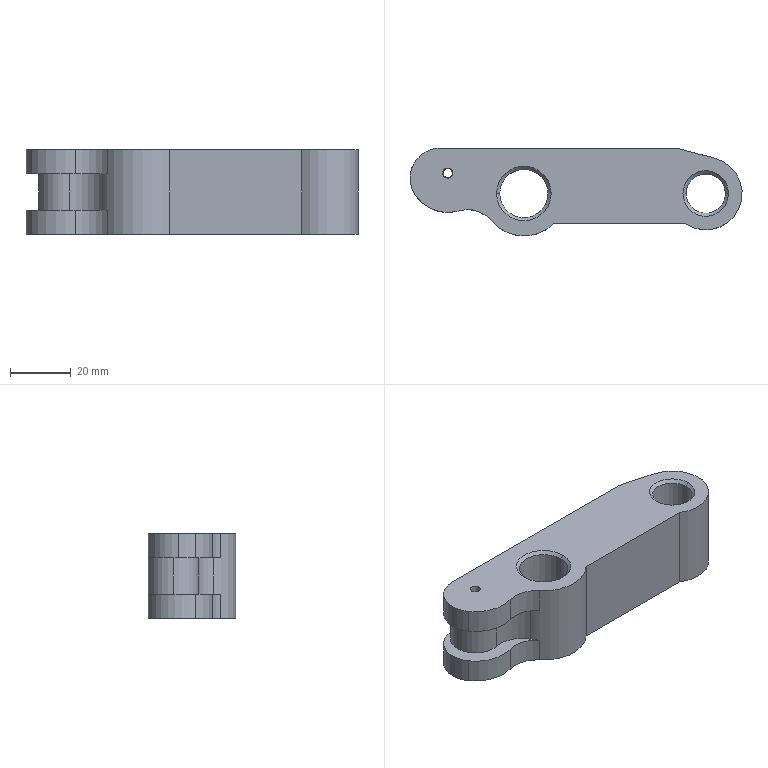Part | SolidWorks | features ICE 3, MirrorPattern 2, 3DProfileFeature 1, Chamfer 1, Extrusion 1, HoleWzd 1 | 1 solid | 45 faces | box 109.566 x 29 x 28 mm | volume 60118 mm3 | cylinder 26 | cone 12 | plane 7 | commonest cylinder face diameters 20 x6 3.3 x4 3.5 x4 3 x2 13 x2 16 x2
STEP:
#1=CARTESIAN_POINT('',(-8.,0.,13.));
#2=VERTEX_POINT('',#1);
#3=CARTESIAN_POINT('',(8.,0.,13.));
#4=VERTEX_POINT('',#3);
#5=CARTESIAN_POINT('',(0.,0.,13.));
#6=DIRECTION('',(0.,0.,1.));
#7=DIRECTION('',(1.,0.,0.));
#8=AXIS2_PLACEMENT_3D('',#5,#6,#7);
#9=CIRCLE('',#8,8.);
#10=EDGE_CURVE('',#2,#4,#9,.T.);
#11=ORIENTED_EDGE('',*,*,#10,.F.);
#12=CARTESIAN_POINT('',(-9.,0.,14.));
#13=VERTEX_POINT('',#12);
#14=CARTESIAN_POINT('',(-8.,0.,13.));
#15=DIRECTION('',(-0.7071,0.,0.7071));
#16=VECTOR('',#15,1000.);
#17=LINE('',#14,#16);
#18=EDGE_CURVE('',#2,#13,#17,.T.);
#19=ORIENTED_EDGE('',*,*,#18,.T.);
#20=CARTESIAN_POINT('',(9.,0.,14.));
#21=VERTEX_POINT('',#20);
#22=CARTESIAN_POINT('',(0.,0.,14.));
#23=DIRECTION('',(0.,0.,-1.));
#24=DIRECTION('',(1.,0.,0.));
#25=AXIS2_PLACEMENT_3D('',#22,#23,#24);
#26=CIRCLE('',#25,9.);
#27=EDGE_CURVE('',#21,#13,#26,.T.);
#28=ORIENTED_EDGE('',*,*,#27,.F.);
#29=CARTESIAN_POINT('',(8.,0.,13.));
#30=DIRECTION('',(0.7071,0.,0.7071));
#31=VECTOR('',#30,1000.);
#32=LINE('',#29,#31);
#33=EDGE_CURVE('',#4,#21,#32,.T.);
#34=ORIENTED_EDGE('',*,*,#33,.F.);
#35=EDGE_LOOP('',(#11,#19,#28,#34));
#36=FACE_OUTER_BOUND('',#35,.T.);
#37=CARTESIAN_POINT('',(0.,0.,13.));
#38=DIRECTION('',(0.,0.,1.));
#39=DIRECTION('',(1.,0.,0.));
#40=AXIS2_PLACEMENT_3D('',#37,#38,#39);
#41=CONICAL_SURFACE('',#40,8.,0.7854);
#42=ADVANCED_FACE('',(#36),#41,.F.);
#43=CARTESIAN_POINT('',(53.5,0.,13.));
#44=VERTEX_POINT('',#43);
#45=CARTESIAN_POINT('',(66.5,0.,13.));
#46=VERTEX_POINT('',#45);
#47=CARTESIAN_POINT('',(60.,0.,13.));
#48=DIRECTION('',(0.,0.,1.));
#49=DIRECTION('',(1.,0.,0.));
#50=AXIS2_PLACEMENT_3D('',#47,#48,#49);
#51=CIRCLE('',#50,6.5);
#52=EDGE_CURVE('',#44,#46,#51,.T.);
#53=ORIENTED_EDGE('',*,*,#52,.F.);
#54=CARTESIAN_POINT('',(52.5,0.,14.));
#55=VERTEX_POINT('',#54);
#56=CARTESIAN_POINT('',(53.5,0.,13.));
#57=DIRECTION('',(-0.7071,0.,0.7071));
#58=VECTOR('',#57,1000.);
#59=LINE('',#56,#58);
#60=EDGE_CURVE('',#44,#55,#59,.T.);
#61=ORIENTED_EDGE('',*,*,#60,.T.);
#62=CARTESIAN_POINT('',(67.5,0.,14.));
#63=VERTEX_POINT('',#62);
#64=CARTESIAN_POINT('',(60.,0.,14.));
#65=DIRECTION('',(0.,0.,-1.));
#66=DIRECTION('',(1.,0.,0.));
#67=AXIS2_PLACEMENT_3D('',#64,#65,#66);
#68=CIRCLE('',#67,7.5);
#69=EDGE_CURVE('',#63,#55,#68,.T.);
#70=ORIENTED_EDGE('',*,*,#69,.F.);
#71=CARTESIAN_POINT('',(66.5,0.,13.));
#72=DIRECTION('',(0.7071,0.,0.7071));
#73=VECTOR('',#72,1000.);
#74=LINE('',#71,#73);
#75=EDGE_CURVE('',#46,#63,#74,.T.);
#76=ORIENTED_EDGE('',*,*,#75,.F.);
#77=EDGE_LOOP('',(#53,#61,#70,#76));
#78=FACE_OUTER_BOUND('',#77,.T.);
#79=CARTESIAN_POINT('',(60.,0.,13.));
#80=DIRECTION('',(0.,0.,1.));
#81=DIRECTION('',(1.,0.,0.));
#82=AXIS2_PLACEMENT_3D('',#79,#80,#81);
#83=CONICAL_SURFACE('',#82,6.5,0.7854);
#84=ADVANCED_FACE('',(#78),#83,.F.);
#85=CARTESIAN_POINT('',(66.5,0.,-13.));
#86=VERTEX_POINT('',#85);
#87=CARTESIAN_POINT('',(53.5,0.,-13.));
#88=VERTEX_POINT('',#87);
#89=CARTESIAN_POINT('',(60.,0.,-13.));
#90=DIRECTION('',(0.,0.,-1.));
#91=DIRECTION('',(-1.,0.,0.));
#92=AXIS2_PLACEMENT_3D('',#89,#90,#91);
#93=CIRCLE('',#92,6.5);
#94=EDGE_CURVE('',#86,#88,#93,.T.);
#95=ORIENTED_EDGE('',*,*,#94,.F.);
#96=CARTESIAN_POINT('',(67.5,0.,-14.));
#97=VERTEX_POINT('',#96);
#98=CARTESIAN_POINT('',(67.5,0.,-14.));
#99=DIRECTION('',(0.7071,0.,-0.7071));
#100=VECTOR('',#99,1000.);
#101=LINE('',#98,#100);
#102=EDGE_CURVE('',#86,#97,#101,.T.);
#103=ORIENTED_EDGE('',*,*,#102,.T.);
#104=CARTESIAN_POINT('',(52.5,0.,-14.));
#105=VERTEX_POINT('',#104);
#106=CARTESIAN_POINT('',(60.,0.,-14.));
#107=DIRECTION('',(0.,0.,1.));
#108=DIRECTION('',(-1.,0.,0.));
#109=AXIS2_PLACEMENT_3D('',#106,#107,#108);
#110=CIRCLE('',#109,7.5);
#111=EDGE_CURVE('',#105,#97,#110,.T.);
#112=ORIENTED_EDGE('',*,*,#111,.F.);
#113=CARTESIAN_POINT('',(52.5,0.,-14.));
#114=DIRECTION('',(-0.7071,0.,-0.7071));
#115=VECTOR('',#114,1000.);
#116=LINE('',#113,#115);
#117=EDGE_CURVE('',#88,#105,#116,.T.);
#118=ORIENTED_EDGE('',*,*,#117,.F.);
#119=EDGE_LOOP('',(#95,#103,#112,#118));
#120=FACE_OUTER_BOUND('',#119,.T.);
#121=CARTESIAN_POINT('',(60.,0.,-14.));
#122=DIRECTION('',(0.,0.,-1.));
#123=DIRECTION('',(-1.,0.,0.));
#124=AXIS2_PLACEMENT_3D('',#121,#122,#123);
#125=CONICAL_SURFACE('',#124,7.5,0.7854);
#126=ADVANCED_FACE('',(#120),#125,.F.);
#127=CARTESIAN_POINT('',(8.,0.,-13.));
#128=VERTEX_POINT('',#127);
#129=CARTESIAN_POINT('',(-8.,0.,-13.));
#130=VERTEX_POINT('',#129);
#131=CARTESIAN_POINT('',(0.,0.,-13.));
#132=DIRECTION('',(0.,0.,-1.));
#133=DIRECTION('',(-1.,0.,0.));
#134=AXIS2_PLACEMENT_3D('',#131,#132,#133);
#135=CIRCLE('',#134,8.);
#136=EDGE_CURVE('',#128,#130,#135,.T.);
#137=ORIENTED_EDGE('',*,*,#136,.F.);
#138=CARTESIAN_POINT('',(9.,0.,-14.));
#139=VERTEX_POINT('',#138);
#140=CARTESIAN_POINT('',(9.,0.,-14.));
#141=DIRECTION('',(0.7071,0.,-0.7071));
#142=VECTOR('',#141,1000.);
#143=LINE('',#140,#142);
#144=EDGE_CURVE('',#128,#139,#143,.T.);
#145=ORIENTED_EDGE('',*,*,#144,.T.);
#146=CARTESIAN_POINT('',(-9.,0.,-14.));
#147=VERTEX_POINT('',#146);
#148=CARTESIAN_POINT('',(0.,0.,-14.));
#149=DIRECTION('',(0.,0.,1.));
#150=DIRECTION('',(-1.,0.,0.));
#151=AXIS2_PLACEMENT_3D('',#148,#149,#150);
#152=CIRCLE('',#151,9.);
#153=EDGE_CURVE('',#147,#139,#152,.T.);
#154=ORIENTED_EDGE('',*,*,#153,.F.);
#155=CARTESIAN_POINT('',(-9.,0.,-14.));
#156=DIRECTION('',(-0.7071,0.,-0.7071));
#157=VECTOR('',#156,1000.);
#158=LINE('',#155,#157);
#159=EDGE_CURVE('',#130,#147,#158,.T.);
#160=ORIENTED_EDGE('',*,*,#159,.F.);
#161=EDGE_LOOP('',(#137,#145,#154,#160));
#162=FACE_OUTER_BOUND('',#161,.T.);
#163=CARTESIAN_POINT('',(0.,0.,-14.));
#164=DIRECTION('',(0.,0.,-1.));
#165=DIRECTION('',(-1.,0.,0.));
#166=AXIS2_PLACEMENT_3D('',#163,#164,#165);
#167=CONICAL_SURFACE('',#166,9.,0.7854);
#168=ADVANCED_FACE('',(#162),#167,.F.);
#169=CARTESIAN_POINT('',(61.75,6.26,-3.));
#170=VERTEX_POINT('',#169);
#171=CARTESIAN_POINT('',(58.25,6.26,-3.));
#172=VERTEX_POINT('',#171);
#173=CARTESIAN_POINT('',(61.75,6.26,-3.));
#174=CARTESIAN_POINT('',(61.75,6.26,-3.229));
#175=CARTESIAN_POINT('',(61.704,6.273,-3.46));
#176=CARTESIAN_POINT('',(61.572,6.307,-3.776));
#177=CARTESIAN_POINT('',(61.518,6.321,-3.879));
#178=CARTESIAN_POINT('',(61.391,6.35,-4.068));
#179=CARTESIAN_POINT('',(61.319,6.365,-4.156));
#180=CARTESIAN_POINT('',(61.157,6.397,-4.318));
#181=CARTESIAN_POINT('',(61.068,6.412,-4.391));
#182=CARTESIAN_POINT('',(60.879,6.441,-4.517));
#183=CARTESIAN_POINT('',(60.779,6.454,-4.571));
#184=CARTESIAN_POINT('',(60.566,6.476,-4.66));
#185=CARTESIAN_POINT('',(60.456,6.485,-4.693));
#186=CARTESIAN_POINT('',(60.232,6.497,-4.738));
#187=CARTESIAN_POINT('',(60.116,6.5,-4.75));
#188=CARTESIAN_POINT('',(59.885,6.5,-4.75));
#189=CARTESIAN_POINT('',(59.771,6.497,-4.739));
#190=CARTESIAN_POINT('',(59.546,6.485,-4.694));
#191=CARTESIAN_POINT('',(59.434,6.476,-4.66));
#192=CARTESIAN_POINT('',(59.118,6.443,-4.529));
#193=CARTESIAN_POINT('',(58.924,6.412,-4.398));
#194=CARTESIAN_POINT('',(58.602,6.35,-4.077));
#195=CARTESIAN_POINT('',(58.472,6.319,-3.884));
#196=CARTESIAN_POINT('',(58.341,6.285,-3.568));
#197=CARTESIAN_POINT('',(58.307,6.276,-3.456));
#198=CARTESIAN_POINT('',(58.261,6.263,-3.231));
#199=CARTESIAN_POINT('',(58.25,6.26,-3.116));
#200=CARTESIAN_POINT('',(58.25,6.26,-3.));
#201=B_SPLINE_CURVE_WITH_KNOTS('',3,(#173,#174,#175,#176,#177,#178,#179,#180,#181,#182,#183,#184,#185,#186,#187,#188,#189,#190,#191,#192,#193,#194,#195,#196,#197,#198,#199,#200),.UNSPECIFIED.,.F.,.F.,(4,2,2,2,2,2,2,2,2,2,2,2,2,4),(0.005497,0.006184,0.006527,0.006871,0.007214,0.007557,0.007901,0.008244,0.008588,0.008931,0.009618,0.01031,0.01065,0.01099),.UNSPECIFIED.);
#202=EDGE_CURVE('',#170,#172,#201,.T.);
#203=ORIENTED_EDGE('',*,*,#202,.F.);
#204=CARTESIAN_POINT('',(61.75,11.954,-3.));
#205=VERTEX_POINT('',#204);
#206=CARTESIAN_POINT('',(61.75,-14.001,-3.));
#207=DIRECTION('',(0.,1.,0.));
#208=VECTOR('',#207,1000.);
#209=LINE('',#206,#208);
#210=EDGE_CURVE('',#170,#205,#209,.T.);
#211=ORIENTED_EDGE('',*,*,#210,.T.);
#212=CARTESIAN_POINT('',(58.25,12.892,-3.));
#213=VERTEX_POINT('',#212);
#214=CARTESIAN_POINT('',(61.75,11.954,-3.));
#215=CARTESIAN_POINT('',(61.75,11.954,-6.5));
#216=CARTESIAN_POINT('',(58.25,12.892,-6.5));
#217=CARTESIAN_POINT('',(58.25,12.892,-3.));
#218=(BOUNDED_CURVE()B_SPLINE_CURVE(3,(#214,#215,#216,#217),.UNSPECIFIED.,.F.,.F.)B_SPLINE_CURVE_WITH_KNOTS((4,4),(3.142,6.283),.UNSPECIFIED.)CURVE()GEOMETRIC_REPRESENTATION_ITEM()RATIONAL_B_SPLINE_CURVE((1.,0.3333,0.3333,1.))REPRESENTATION_ITEM(''));
#219=EDGE_CURVE('',#205,#213,#218,.T.);
#220=ORIENTED_EDGE('',*,*,#219,.T.);
#221=CARTESIAN_POINT('',(58.25,-14.001,-3.));
#222=DIRECTION('',(0.,1.,0.));
#223=VECTOR('',#222,1000.);
#224=LINE('',#221,#223);
#225=EDGE_CURVE('',#172,#213,#224,.T.);
#226=ORIENTED_EDGE('',*,*,#225,.F.);
#227=EDGE_LOOP('',(#203,#211,#220,#226));
#228=FACE_OUTER_BOUND('',#227,.T.);
#229=CARTESIAN_POINT('',(60.,-14.001,-3.));
#230=DIRECTION('',(0.,1.,0.));
#231=DIRECTION('',(-1.,0.,0.));
#232=AXIS2_PLACEMENT_3D('',#229,#230,#231);
#233=CYLINDRICAL_SURFACE('',#232,1.75);
#234=ADVANCED_FACE('',(#228),#233,.F.);
#235=CARTESIAN_POINT('',(1.75,7.806,0.));
#236=VERTEX_POINT('',#235);
#237=CARTESIAN_POINT('',(-1.75,7.806,0.));
#238=VERTEX_POINT('',#237);
#239=CARTESIAN_POINT('',(1.75,7.806,0.));
#240=CARTESIAN_POINT('',(1.75,7.806,-0.2288));
#241=CARTESIAN_POINT('',(1.704,7.817,-0.4597));
#242=CARTESIAN_POINT('',(1.573,7.844,-0.7757));
#243=CARTESIAN_POINT('',(1.518,7.855,-0.8779));
#244=CARTESIAN_POINT('',(1.391,7.878,-1.068));
#245=CARTESIAN_POINT('',(1.319,7.891,-1.156));
#246=CARTESIAN_POINT('',(1.158,7.916,-1.317));
#247=CARTESIAN_POINT('',(1.068,7.929,-1.391));
#248=CARTESIAN_POINT('',(0.8785,7.952,-1.518));
#249=CARTESIAN_POINT('',(0.7782,7.963,-1.572));
#250=CARTESIAN_POINT('',(0.4594,7.99,-1.704));
#251=CARTESIAN_POINT('',(0.2317,8.,-1.75));
#252=CARTESIAN_POINT('',(-0.1147,8.,-1.75));
#253=CARTESIAN_POINT('',(-0.2286,7.998,-1.739));
#254=CARTESIAN_POINT('',(-0.453,7.988,-1.694));
#255=CARTESIAN_POINT('',(-0.5647,7.981,-1.66));
#256=CARTESIAN_POINT('',(-0.8816,7.954,-1.529));
#257=CARTESIAN_POINT('',(-1.076,7.929,-1.399));
#258=CARTESIAN_POINT('',(-1.398,7.879,-1.077));
#259=CARTESIAN_POINT('',(-1.528,7.853,-0.883));
#260=CARTESIAN_POINT('',(-1.659,7.826,-0.5673));
#261=CARTESIAN_POINT('',(-1.693,7.819,-0.4561));
#262=CARTESIAN_POINT('',(-1.739,7.809,-0.2304));
#263=CARTESIAN_POINT('',(-1.75,7.806,-0.116));
#264=CARTESIAN_POINT('',(-1.75,7.806,0.));
#265=B_SPLINE_CURVE_WITH_KNOTS('',3,(#239,#240,#241,#242,#243,#244,#245,#246,#247,#248,#249,#250,#251,#252,#253,#254,#255,#256,#257,#258,#259,#260,#261,#262,#263,#264),.UNSPECIFIED.,.F.,.F.,(4,2,2,2,2,2,2,2,2,2,2,2,4),(0.005488,0.006174,0.006517,0.00686,0.007202,0.007545,0.008231,0.008574,0.008917,0.009603,0.01029,0.01063,0.01097),.UNSPECIFIED.);
#266=EDGE_CURVE('',#236,#238,#265,.T.);
#267=ORIENTED_EDGE('',*,*,#266,.F.);
#268=CARTESIAN_POINT('',(1.75,15.,0.));
#269=VERTEX_POINT('',#268);
#270=CARTESIAN_POINT('',(1.75,-14.001,0.));
#271=DIRECTION('',(0.,1.,0.));
#272=VECTOR('',#271,1000.);
#273=LINE('',#270,#272);
#274=EDGE_CURVE('',#236,#269,#273,.T.);
#275=ORIENTED_EDGE('',*,*,#274,.T.);
#276=CARTESIAN_POINT('',(-1.75,15.,0.));
#277=VERTEX_POINT('',#276);
#278=CARTESIAN_POINT('',(0.,15.,0.));
#279=DIRECTION('',(0.,1.,0.));
#280=DIRECTION('',(-1.,0.,0.));
#281=AXIS2_PLACEMENT_3D('',#278,#279,#280);
#282=CIRCLE('',#281,1.75);
#283=EDGE_CURVE('',#269,#277,#282,.T.);
#284=ORIENTED_EDGE('',*,*,#283,.T.);
#285=CARTESIAN_POINT('',(-1.75,-14.001,0.));
#286=DIRECTION('',(0.,1.,0.));
#287=VECTOR('',#286,1000.);
#288=LINE('',#285,#287);
#289=EDGE_CURVE('',#238,#277,#288,.T.);
#290=ORIENTED_EDGE('',*,*,#289,.F.);
#291=EDGE_LOOP('',(#267,#275,#284,#290));
#292=FACE_OUTER_BOUND('',#291,.T.);
#293=CARTESIAN_POINT('',(0.,-14.001,0.));
#294=DIRECTION('',(0.,1.,0.));
#295=DIRECTION('',(-1.,0.,0.));
#296=AXIS2_PLACEMENT_3D('',#293,#294,#295);
#297=CYLINDRICAL_SURFACE('',#296,1.75);
#298=ADVANCED_FACE('',(#292),#297,.F.);
#299=CARTESIAN_POINT('',(-23.464,6.729,-6.));
#300=VERTEX_POINT('',#299);
#301=CARTESIAN_POINT('',(-26.764,6.729,-6.));
#302=VERTEX_POINT('',#301);
#303=CARTESIAN_POINT('',(-25.114,6.729,-6.));
#304=DIRECTION('',(0.,0.,-1.));
#305=DIRECTION('',(-1.,0.,0.));
#306=AXIS2_PLACEMENT_3D('',#303,#304,#305);
#307=CIRCLE('',#306,1.65);
#308=EDGE_CURVE('',#300,#302,#307,.T.);
#309=ORIENTED_EDGE('',*,*,#308,.F.);
#310=CARTESIAN_POINT('',(-23.464,6.729,-14.));
#311=VERTEX_POINT('',#310);
#312=CARTESIAN_POINT('',(-23.464,6.729,-14.));
#313=DIRECTION('',(0.,0.,-1.));
#314=VECTOR('',#313,1000.);
#315=LINE('',#312,#314);
#316=EDGE_CURVE('',#300,#311,#315,.T.);
#317=ORIENTED_EDGE('',*,*,#316,.T.);
#318=CARTESIAN_POINT('',(-26.764,6.729,-14.));
#319=VERTEX_POINT('',#318);
#320=CARTESIAN_POINT('',(-25.114,6.729,-14.));
#321=DIRECTION('',(0.,0.,-1.));
#322=DIRECTION('',(-1.,0.,0.));
#323=AXIS2_PLACEMENT_3D('',#320,#321,#322);
#324=CIRCLE('',#323,1.65);
#325=EDGE_CURVE('',#311,#319,#324,.T.);
#326=ORIENTED_EDGE('',*,*,#325,.T.);
#327=CARTESIAN_POINT('',(-26.764,6.729,-14.));
#328=DIRECTION('',(0.,0.,-1.));
#329=VECTOR('',#328,1000.);
#330=LINE('',#327,#329);
#331=EDGE_CURVE('',#302,#319,#330,.T.);
#332=ORIENTED_EDGE('',*,*,#331,.F.);
#333=EDGE_LOOP('',(#309,#317,#326,#332));
#334=FACE_OUTER_BOUND('',#333,.T.);
#335=CARTESIAN_POINT('',(-25.114,6.729,-14.));
#336=DIRECTION('',(0.,0.,-1.));
#337=DIRECTION('',(-1.,0.,0.));
#338=AXIS2_PLACEMENT_3D('',#335,#336,#337);
#339=CYLINDRICAL_SURFACE('',#338,1.65);
#340=ADVANCED_FACE('',(#334),#339,.F.);
#341=CARTESIAN_POINT('',(-26.614,6.729,-5.91));
#342=VERTEX_POINT('',#341);
#343=CARTESIAN_POINT('',(-23.614,6.729,-5.91));
#344=VERTEX_POINT('',#343);
#345=CARTESIAN_POINT('',(-25.114,6.729,-5.91));
#346=DIRECTION('',(0.,0.,1.));
#347=DIRECTION('',(-1.,0.,0.));
#348=AXIS2_PLACEMENT_3D('',#345,#346,#347);
#349=CIRCLE('',#348,1.5);
#350=EDGE_CURVE('',#342,#344,#349,.T.);
#351=ORIENTED_EDGE('',*,*,#350,.T.);
#352=CARTESIAN_POINT('',(-23.464,6.729,-6.));
#353=DIRECTION('',(0.8572,0.,-0.515));
#354=VECTOR('',#353,1000.);
#355=LINE('',#352,#354);
#356=EDGE_CURVE('',#344,#300,#355,.T.);
#357=ORIENTED_EDGE('',*,*,#356,.T.);
#358=ORIENTED_EDGE('',*,*,#308,.T.);
#359=CARTESIAN_POINT('',(-26.764,6.729,-6.));
#360=DIRECTION('',(-0.8572,0.,-0.515));
#361=VECTOR('',#360,1000.);
#362=LINE('',#359,#361);
#363=EDGE_CURVE('',#342,#302,#362,.T.);
#364=ORIENTED_EDGE('',*,*,#363,.F.);
#365=EDGE_LOOP('',(#351,#357,#358,#364));
#366=FACE_OUTER_BOUND('',#365,.T.);
#367=CARTESIAN_POINT('',(-25.114,6.729,-6.));
#368=DIRECTION('',(0.,0.,-1.));
#369=DIRECTION('',(-1.,0.,0.));
#370=AXIS2_PLACEMENT_3D('',#367,#368,#369);
#371=CONICAL_SURFACE('',#370,1.65,1.03);
#372=ADVANCED_FACE('',(#366),#371,.F.);
#373=CARTESIAN_POINT('',(-37.566,5.,14.));
#374=VERTEX_POINT('',#373);
#375=CARTESIAN_POINT('',(-35.738,-0.763,14.));
#376=VERTEX_POINT('',#375);
#377=CARTESIAN_POINT('',(-27.566,5.,14.));
#378=DIRECTION('',(0.,0.,1.));
#379=DIRECTION('',(1.,0.,0.));
#380=AXIS2_PLACEMENT_3D('',#377,#378,#379);
#381=CIRCLE('',#380,10.);
#382=EDGE_CURVE('',#374,#376,#381,.T.);
#383=ORIENTED_EDGE('',*,*,#382,.F.);
#384=CARTESIAN_POINT('',(-37.566,5.,6.));
#385=VERTEX_POINT('',#384);
#386=CARTESIAN_POINT('',(-37.566,5.,14.));
#387=DIRECTION('',(0.,0.,-1.));
#388=VECTOR('',#387,1000.);
#389=LINE('',#386,#388);
#390=EDGE_CURVE('',#374,#385,#389,.T.);
#391=ORIENTED_EDGE('',*,*,#390,.T.);
#392=CARTESIAN_POINT('',(-35.738,-0.763,6.));
#393=VERTEX_POINT('',#392);
#394=CARTESIAN_POINT('',(-27.566,5.,6.));
#395=DIRECTION('',(0.,0.,1.));
#396=DIRECTION('',(1.,0.,0.));
#397=AXIS2_PLACEMENT_3D('',#394,#395,#396);
#398=CIRCLE('',#397,10.);
#399=EDGE_CURVE('',#385,#393,#398,.T.);
#400=ORIENTED_EDGE('',*,*,#399,.T.);
#401=CARTESIAN_POINT('',(-35.738,-0.763,14.));
#402=DIRECTION('',(0.,0.,-1.));
#403=VECTOR('',#402,1000.);
#404=LINE('',#401,#403);
#405=EDGE_CURVE('',#376,#393,#404,.T.);
#406=ORIENTED_EDGE('',*,*,#405,.F.);
#407=EDGE_LOOP('',(#383,#391,#400,#406));
#408=FACE_OUTER_BOUND('',#407,.T.);
#409=CARTESIAN_POINT('',(-27.566,5.,14.));
#410=DIRECTION('',(0.,0.,-1.));
#411=DIRECTION('',(-1.,0.,0.));
#412=AXIS2_PLACEMENT_3D('',#409,#410,#411);
#413=CYLINDRICAL_SURFACE('',#412,10.);
#414=ADVANCED_FACE('',(#408),#413,.T.);
#415=ORIENTED_EDGE('',*,*,#52,.T.);
#416=CARTESIAN_POINT('',(66.5,0.,6.));
#417=DIRECTION('',(0.,0.,-1.));
#418=VECTOR('',#417,1000.);
#419=LINE('',#416,#418);
#420=EDGE_CURVE('',#46,#86,#419,.T.);
#421=ORIENTED_EDGE('',*,*,#420,.T.);
#422=ORIENTED_EDGE('',*,*,#94,.T.);
#423=CARTESIAN_POINT('',(53.5,0.,6.));
#424=DIRECTION('',(0.,0.,-1.));
#425=VECTOR('',#424,1000.);
#426=LINE('',#423,#425);
#427=EDGE_CURVE('',#44,#88,#426,.T.);
#428=ORIENTED_EDGE('',*,*,#427,.F.);
#429=EDGE_LOOP('',(#415,#421,#422,#428));
#430=FACE_OUTER_BOUND('',#429,.T.);
#431=CARTESIAN_POINT('',(60.,0.,6.));
#432=DIRECTION('',(0.,0.,-1.));
#433=DIRECTION('',(-1.,0.,0.));
#434=AXIS2_PLACEMENT_3D('',#431,#432,#433);
#435=CYLINDRICAL_SURFACE('',#434,6.5);
#436=ADVANCED_FACE('',(#430),#435,.F.);
#437=ORIENTED_EDGE('',*,*,#10,.T.);
#438=CARTESIAN_POINT('',(8.,0.,6.));
#439=DIRECTION('',(0.,0.,-1.));
#440=VECTOR('',#439,1000.);
#441=LINE('',#438,#440);
#442=EDGE_CURVE('',#4,#128,#441,.T.);
#443=ORIENTED_EDGE('',*,*,#442,.T.);
#444=ORIENTED_EDGE('',*,*,#136,.T.);
#445=CARTESIAN_POINT('',(-8.,0.,6.));
#446=DIRECTION('',(0.,0.,-1.));
#447=VECTOR('',#446,1000.);
#448=LINE('',#445,#447);
#449=EDGE_CURVE('',#2,#130,#448,.T.);
#450=ORIENTED_EDGE('',*,*,#449,.F.);
#451=EDGE_LOOP('',(#437,#443,#444,#450));
#452=FACE_OUTER_BOUND('',#451,.T.);
#453=CARTESIAN_POINT('',(0.,0.,6.));
#454=DIRECTION('',(0.,0.,-1.));
#455=DIRECTION('',(-1.,0.,0.));
#456=AXIS2_PLACEMENT_3D('',#453,#454,#455);
#457=CYLINDRICAL_SURFACE('',#456,8.);
#458=ADVANCED_FACE('',(#452),#457,.F.);
#459=CARTESIAN_POINT('',(-33.385,6.729,6.));
#460=VERTEX_POINT('',#459);
#461=CARTESIAN_POINT('',(-23.371,-1.356,6.));
#462=VERTEX_POINT('',#461);
#463=CARTESIAN_POINT('',(-25.114,6.729,6.));
#464=DIRECTION('',(0.,0.,1.));
#465=DIRECTION('',(1.,0.,0.));
#466=AXIS2_PLACEMENT_3D('',#463,#464,#465);
#467=CIRCLE('',#466,8.271);
#468=EDGE_CURVE('',#460,#462,#467,.T.);
#469=ORIENTED_EDGE('',*,*,#468,.F.);
#470=CARTESIAN_POINT('',(-33.385,6.729,-6.));
#471=VERTEX_POINT('',#470);
#472=CARTESIAN_POINT('',(-33.385,6.729,6.));
#473=DIRECTION('',(0.,0.,-1.));
#474=VECTOR('',#473,1000.);
#475=LINE('',#472,#474);
#476=EDGE_CURVE('',#460,#471,#475,.T.);
#477=ORIENTED_EDGE('',*,*,#476,.T.);
#478=CARTESIAN_POINT('',(-23.371,-1.356,-6.));
#479=VERTEX_POINT('',#478);
#480=CARTESIAN_POINT('',(-25.114,6.729,-6.));
#481=DIRECTION('',(0.,0.,1.));
#482=DIRECTION('',(1.,0.,0.));
#483=AXIS2_PLACEMENT_3D('',#480,#481,#482);
#484=CIRCLE('',#483,8.271);
#485=EDGE_CURVE('',#471,#479,#484,.T.);
#486=ORIENTED_EDGE('',*,*,#485,.T.);
#487=CARTESIAN_POINT('',(-23.371,-1.356,6.));
#488=DIRECTION('',(0.,0.,-1.));
#489=VECTOR('',#488,1000.);
#490=LINE('',#487,#489);
#491=EDGE_CURVE('',#462,#479,#490,.T.);
#492=ORIENTED_EDGE('',*,*,#491,.F.);
#493=EDGE_LOOP('',(#469,#477,#486,#492));
#494=FACE_OUTER_BOUND('',#493,.T.);
#495=CARTESIAN_POINT('',(-25.114,6.729,6.));
#496=DIRECTION('',(0.,0.,-1.));
#497=DIRECTION('',(-1.,0.,0.));
#498=AXIS2_PLACEMENT_3D('',#495,#496,#497);
#499=CYLINDRICAL_SURFACE('',#498,8.271);
#500=ADVANCED_FACE('',(#494),#499,.T.);
#501=CARTESIAN_POINT('',(-26.764,6.729,6.));
#502=VERTEX_POINT('',#501);
#503=CARTESIAN_POINT('',(-23.464,6.729,6.));
#504=VERTEX_POINT('',#503);
#505=CARTESIAN_POINT('',(-25.114,6.729,6.));
#506=DIRECTION('',(0.,0.,1.));
#507=DIRECTION('',(1.,0.,0.));
#508=AXIS2_PLACEMENT_3D('',#505,#506,#507);
#509=CIRCLE('',#508,1.65);
#510=EDGE_CURVE('',#502,#504,#509,.T.);
#511=ORIENTED_EDGE('',*,*,#510,.F.);
#512=CARTESIAN_POINT('',(-26.764,6.729,14.));
#513=VERTEX_POINT('',#512);
#514=CARTESIAN_POINT('',(-26.764,6.729,14.));
#515=DIRECTION('',(0.,0.,1.));
#516=VECTOR('',#515,1000.);
#517=LINE('',#514,#516);
#518=EDGE_CURVE('',#502,#513,#517,.T.);
#519=ORIENTED_EDGE('',*,*,#518,.T.);
#520=CARTESIAN_POINT('',(-23.464,6.729,14.));
#521=VERTEX_POINT('',#520);
#522=CARTESIAN_POINT('',(-25.114,6.729,14.));
#523=DIRECTION('',(0.,0.,1.));
#524=DIRECTION('',(1.,0.,0.));
#525=AXIS2_PLACEMENT_3D('',#522,#523,#524);
#526=CIRCLE('',#525,1.65);
#527=EDGE_CURVE('',#513,#521,#526,.T.);
#528=ORIENTED_EDGE('',*,*,#527,.T.);
#529=CARTESIAN_POINT('',(-23.464,6.729,14.));
#530=DIRECTION('',(0.,0.,1.));
#531=VECTOR('',#530,1000.);
#532=LINE('',#529,#531);
#533=EDGE_CURVE('',#504,#521,#532,.T.);
#534=ORIENTED_EDGE('',*,*,#533,.F.);
#535=EDGE_LOOP('',(#511,#519,#528,#534));
#536=FACE_OUTER_BOUND('',#535,.T.);
#537=CARTESIAN_POINT('',(-25.114,6.729,14.));
#538=DIRECTION('',(0.,0.,1.));
#539=DIRECTION('',(1.,0.,0.));
#540=AXIS2_PLACEMENT_3D('',#537,#538,#539);
#541=CYLINDRICAL_SURFACE('',#540,1.65);
#542=ADVANCED_FACE('',(#536),#541,.F.);
#543=CARTESIAN_POINT('',(-23.614,6.729,5.91));
#544=VERTEX_POINT('',#543);
#545=CARTESIAN_POINT('',(-26.614,6.729,5.91));
#546=VERTEX_POINT('',#545);
#547=CARTESIAN_POINT('',(-25.114,6.729,5.91));
#548=DIRECTION('',(0.,0.,-1.));
#549=DIRECTION('',(1.,0.,0.));
#550=AXIS2_PLACEMENT_3D('',#547,#548,#549);
#551=CIRCLE('',#550,1.5);
#552=EDGE_CURVE('',#544,#546,#551,.T.);
#553=ORIENTED_EDGE('',*,*,#552,.T.);
#554=CARTESIAN_POINT('',(-26.764,6.729,6.));
#555=DIRECTION('',(-0.8572,0.,0.515));
#556=VECTOR('',#555,1000.);
#557=LINE('',#554,#556);
#558=EDGE_CURVE('',#546,#502,#557,.T.);
#559=ORIENTED_EDGE('',*,*,#558,.T.);
#560=ORIENTED_EDGE('',*,*,#510,.T.);
#561=CARTESIAN_POINT('',(-23.464,6.729,6.));
#562=DIRECTION('',(0.8572,0.,0.515));
#563=VECTOR('',#562,1000.);
#564=LINE('',#561,#563);
#565=EDGE_CURVE('',#544,#504,#564,.T.);
#566=ORIENTED_EDGE('',*,*,#565,.F.);
#567=EDGE_LOOP('',(#553,#559,#560,#566));
#568=FACE_OUTER_BOUND('',#567,.T.);
#569=CARTESIAN_POINT('',(-25.114,6.729,6.));
#570=DIRECTION('',(0.,0.,1.));
#571=DIRECTION('',(1.,0.,0.));
#572=AXIS2_PLACEMENT_3D('',#569,#570,#571);
#573=CONICAL_SURFACE('',#572,1.65,1.03);
#574=ADVANCED_FACE('',(#568),#573,.F.);
#575=ORIENTED_EDGE('',*,*,#552,.F.);
#576=CARTESIAN_POINT('',(-23.614,6.729,6.));
#577=DIRECTION('',(0.,0.,-1.));
#578=VECTOR('',#577,1000.);
#579=LINE('',#576,#578);
#580=EDGE_CURVE('',#544,#344,#579,.T.);
#581=ORIENTED_EDGE('',*,*,#580,.T.);
#582=ORIENTED_EDGE('',*,*,#350,.F.);
#583=CARTESIAN_POINT('',(-26.614,6.729,6.));
#584=DIRECTION('',(0.,0.,-1.));
#585=VECTOR('',#584,1000.);
#586=LINE('',#583,#585);
#587=EDGE_CURVE('',#546,#342,#586,.T.);
#588=ORIENTED_EDGE('',*,*,#587,.F.);
#589=EDGE_LOOP('',(#575,#581,#582,#588));
#590=FACE_OUTER_BOUND('',#589,.T.);
#591=CARTESIAN_POINT('',(-25.114,6.729,6.));
#592=DIRECTION('',(0.,0.,-1.));
#593=DIRECTION('',(-1.,0.,0.));
#594=AXIS2_PLACEMENT_3D('',#591,#592,#593);
#595=CYLINDRICAL_SURFACE('',#594,1.5);
#596=ADVANCED_FACE('',(#590),#595,.F.);
#597=ORIENTED_EDGE('',*,*,#580,.F.);
#598=CARTESIAN_POINT('',(-25.114,6.729,5.91));
#599=DIRECTION('',(0.,0.,-1.));
#600=DIRECTION('',(1.,0.,0.));
#601=AXIS2_PLACEMENT_3D('',#598,#599,#600);
#602=CIRCLE('',#601,1.5);
#603=EDGE_CURVE('',#546,#544,#602,.T.);
#604=ORIENTED_EDGE('',*,*,#603,.F.);
#605=ORIENTED_EDGE('',*,*,#587,.T.);
#606=CARTESIAN_POINT('',(-25.114,6.729,-5.91));
#607=DIRECTION('',(0.,0.,1.));
#608=DIRECTION('',(-1.,0.,0.));
#609=AXIS2_PLACEMENT_3D('',#606,#607,#608);
#610=CIRCLE('',#609,1.5);
#611=EDGE_CURVE('',#344,#342,#610,.T.);
#612=ORIENTED_EDGE('',*,*,#611,.F.);
#613=EDGE_LOOP('',(#597,#604,#605,#612));
#614=FACE_OUTER_BOUND('',#613,.T.);
#615=CARTESIAN_POINT('',(-25.114,6.729,6.));
#616=DIRECTION('',(0.,0.,-1.));
#617=DIRECTION('',(-1.,0.,0.));
#618=AXIS2_PLACEMENT_3D('',#615,#616,#617);
#619=CYLINDRICAL_SURFACE('',#618,1.5);
#620=ADVANCED_FACE('',(#614),#619,.F.);
#621=ORIENTED_EDGE('',*,*,#558,.F.);
#622=ORIENTED_EDGE('',*,*,#603,.T.);
#623=ORIENTED_EDGE('',*,*,#565,.T.);
#624=CARTESIAN_POINT('',(-25.114,6.729,6.));
#625=DIRECTION('',(0.,0.,1.));
#626=DIRECTION('',(1.,0.,0.));
#627=AXIS2_PLACEMENT_3D('',#624,#625,#626);
#628=CIRCLE('',#627,1.65);
#629=EDGE_CURVE('',#504,#502,#628,.T.);
#630=ORIENTED_EDGE('',*,*,#629,.T.);
#631=EDGE_LOOP('',(#621,#622,#623,#630));
#632=FACE_OUTER_BOUND('',#631,.T.);
#633=CARTESIAN_POINT('',(-25.114,6.729,6.));
#634=DIRECTION('',(0.,0.,1.));
#635=DIRECTION('',(1.,0.,0.));
#636=AXIS2_PLACEMENT_3D('',#633,#634,#635);
#637=CONICAL_SURFACE('',#636,1.65,1.03);
#638=ADVANCED_FACE('',(#632),#637,.F.);
#639=ORIENTED_EDGE('',*,*,#518,.F.);
#640=ORIENTED_EDGE('',*,*,#629,.F.);
#641=ORIENTED_EDGE('',*,*,#533,.T.);
#642=CARTESIAN_POINT('',(-25.114,6.729,14.));
#643=DIRECTION('',(0.,0.,1.));
#644=DIRECTION('',(1.,0.,0.));
#645=AXIS2_PLACEMENT_3D('',#642,#643,#644);
#646=CIRCLE('',#645,1.65);
#647=EDGE_CURVE('',#521,#513,#646,.T.);
#648=ORIENTED_EDGE('',*,*,#647,.T.);
#649=EDGE_LOOP('',(#639,#640,#641,#648));
#650=FACE_OUTER_BOUND('',#649,.T.);
#651=CARTESIAN_POINT('',(-25.114,6.729,14.));
#652=DIRECTION('',(0.,0.,1.));
#653=DIRECTION('',(1.,0.,0.));
#654=AXIS2_PLACEMENT_3D('',#651,#652,#653);
#655=CYLINDRICAL_SURFACE('',#654,1.65);
#656=ADVANCED_FACE('',(#650),#655,.F.);
#657=CARTESIAN_POINT('',(-12.403,-6.493,-6.));
#658=VERTEX_POINT('',#657);
#659=CARTESIAN_POINT('',(-21.263,-11.131,-6.));
#660=DIRECTION('',(0.,0.,-1.));
#661=DIRECTION('',(1.,0.,0.));
#662=AXIS2_PLACEMENT_3D('',#659,#660,#661);
#663=CIRCLE('',#662,10.);
#664=EDGE_CURVE('',#479,#658,#663,.T.);
#665=ORIENTED_EDGE('',*,*,#664,.T.);
#666=CARTESIAN_POINT('',(-12.403,-6.493,6.));
#667=VERTEX_POINT('',#666);
#668=CARTESIAN_POINT('',(-12.403,-6.493,6.));
#669=DIRECTION('',(0.,0.,-1.));
#670=VECTOR('',#669,1000.);
#671=LINE('',#668,#670);
#672=EDGE_CURVE('',#667,#658,#671,.T.);
#673=ORIENTED_EDGE('',*,*,#672,.F.);
#674=CARTESIAN_POINT('',(-21.263,-11.131,6.));
#675=DIRECTION('',(0.,0.,-1.));
#676=DIRECTION('',(1.,0.,0.));
#677=AXIS2_PLACEMENT_3D('',#674,#675,#676);
#678=CIRCLE('',#677,10.);
#679=EDGE_CURVE('',#462,#667,#678,.T.);
#680=ORIENTED_EDGE('',*,*,#679,.F.);
#681=ORIENTED_EDGE('',*,*,#491,.T.);
#682=EDGE_LOOP('',(#665,#673,#680,#681));
#683=FACE_OUTER_BOUND('',#682,.T.);
#684=CARTESIAN_POINT('',(-21.263,-11.131,6.));
#685=DIRECTION('',(0.,0.,-1.));
#686=DIRECTION('',(-1.,0.,0.));
#687=AXIS2_PLACEMENT_3D('',#684,#685,#686);
#688=CYLINDRICAL_SURFACE('',#687,10.);
#689=ADVANCED_FACE('',(#683),#688,.F.);
#690=CARTESIAN_POINT('',(-10.788,-8.923,-6.));
#691=VERTEX_POINT('',#690);
#692=CARTESIAN_POINT('',(0.,0.,-6.));
#693=DIRECTION('',(0.,0.,1.));
#694=DIRECTION('',(1.,0.,0.));
#695=AXIS2_PLACEMENT_3D('',#692,#693,#694);
#696=CIRCLE('',#695,14.);
#697=EDGE_CURVE('',#658,#691,#696,.T.);
#698=ORIENTED_EDGE('',*,*,#697,.T.);
#699=CARTESIAN_POINT('',(-10.788,-8.923,-14.));
#700=VERTEX_POINT('',#699);
#701=CARTESIAN_POINT('',(-10.788,-8.923,-14.));
#702=DIRECTION('',(0.,0.,1.));
#703=VECTOR('',#702,1000.);
#704=LINE('',#701,#703);
#705=EDGE_CURVE('',#700,#691,#704,.T.);
#706=ORIENTED_EDGE('',*,*,#705,.F.);
#707=CARTESIAN_POINT('',(9.798,-10.,-14.));
#708=VERTEX_POINT('',#707);
#709=CARTESIAN_POINT('',(0.,0.,-14.));
#710=DIRECTION('',(0.,0.,1.));
#711=DIRECTION('',(1.,0.,0.));
#712=AXIS2_PLACEMENT_3D('',#709,#710,#711);
#713=CIRCLE('',#712,14.);
#714=EDGE_CURVE('',#700,#708,#713,.T.);
#715=ORIENTED_EDGE('',*,*,#714,.T.);
#716=CARTESIAN_POINT('',(9.798,-10.,14.));
#717=VERTEX_POINT('',#716);
#718=CARTESIAN_POINT('',(9.798,-10.,6.));
#719=DIRECTION('',(0.,0.,-1.));
#720=VECTOR('',#719,1000.);
#721=LINE('',#718,#720);
#722=EDGE_CURVE('',#717,#708,#721,.T.);
#723=ORIENTED_EDGE('',*,*,#722,.F.);
#724=CARTESIAN_POINT('',(-10.788,-8.923,14.));
#725=VERTEX_POINT('',#724);
#726=CARTESIAN_POINT('',(0.,0.,14.));
#727=DIRECTION('',(0.,0.,1.));
#728=DIRECTION('',(1.,0.,0.));
#729=AXIS2_PLACEMENT_3D('',#726,#727,#728);
#730=CIRCLE('',#729,14.);
#731=EDGE_CURVE('',#725,#717,#730,.T.);
#732=ORIENTED_EDGE('',*,*,#731,.F.);
#733=CARTESIAN_POINT('',(-10.788,-8.923,6.));
#734=VERTEX_POINT('',#733);
#735=CARTESIAN_POINT('',(-10.788,-8.923,14.));
#736=DIRECTION('',(0.,0.,-1.));
#737=VECTOR('',#736,1000.);
#738=LINE('',#735,#737);
#739=EDGE_CURVE('',#725,#734,#738,.T.);
#740=ORIENTED_EDGE('',*,*,#739,.T.);
#741=CARTESIAN_POINT('',(0.,0.,6.));
#742=DIRECTION('',(0.,0.,1.));
#743=DIRECTION('',(1.,0.,0.));
#744=AXIS2_PLACEMENT_3D('',#741,#742,#743);
#745=CIRCLE('',#744,14.);
#746=EDGE_CURVE('',#667,#734,#745,.T.);
#747=ORIENTED_EDGE('',*,*,#746,.F.);
#748=ORIENTED_EDGE('',*,*,#672,.T.);
#749=EDGE_LOOP('',(#698,#706,#715,#723,#732,#740,#747,#748));
#750=FACE_OUTER_BOUND('',#749,.T.);
#751=CARTESIAN_POINT('',(0.,0.,6.));
#752=DIRECTION('',(0.,0.,-1.));
#753=DIRECTION('',(-1.,0.,0.));
#754=AXIS2_PLACEMENT_3D('',#751,#752,#753);
#755=CYLINDRICAL_SURFACE('',#754,14.);
#756=ADVANCED_FACE('',(#750),#755,.T.);
#757=ORIENTED_EDGE('',*,*,#722,.T.);
#758=CARTESIAN_POINT('',(53.367,-10.,-14.));
#759=VERTEX_POINT('',#758);
#760=CARTESIAN_POINT('',(9.798,-10.,-14.));
#761=DIRECTION('',(1.,0.,0.));
#762=VECTOR('',#761,1000.);
#763=LINE('',#760,#762);
#764=EDGE_CURVE('',#708,#759,#763,.T.);
#765=ORIENTED_EDGE('',*,*,#764,.T.);
#766=CARTESIAN_POINT('',(53.367,-10.,14.));
#767=VERTEX_POINT('',#766);
#768=CARTESIAN_POINT('',(53.367,-10.,6.));
#769=DIRECTION('',(0.,0.,-1.));
#770=VECTOR('',#769,1000.);
#771=LINE('',#768,#770);
#772=EDGE_CURVE('',#767,#759,#771,.T.);
#773=ORIENTED_EDGE('',*,*,#772,.F.);
#774=CARTESIAN_POINT('',(9.798,-10.,14.));
#775=DIRECTION('',(1.,0.,0.));
#776=VECTOR('',#775,1000.);
#777=LINE('',#774,#776);
#778=EDGE_CURVE('',#717,#767,#777,.T.);
#779=ORIENTED_EDGE('',*,*,#778,.F.);
#780=EDGE_LOOP('',(#757,#765,#773,#779));
#781=FACE_OUTER_BOUND('',#780,.T.);
#782=CARTESIAN_POINT('',(9.798,-10.,6.));
#783=DIRECTION('',(0.,1.,0.));
#784=DIRECTION('',(0.,0.,1.));
#785=AXIS2_PLACEMENT_3D('',#782,#783,#784);
#786=PLANE('',#785);
#787=ADVANCED_FACE('',(#781),#786,.F.);
#788=ORIENTED_EDGE('',*,*,#772,.T.);
#789=CARTESIAN_POINT('',(63.106,11.591,-14.));
#790=VERTEX_POINT('',#789);
#791=CARTESIAN_POINT('',(60.,0.,-14.));
#792=DIRECTION('',(0.,0.,1.));
#793=DIRECTION('',(1.,0.,0.));
#794=AXIS2_PLACEMENT_3D('',#791,#792,#793);
#795=CIRCLE('',#794,12.);
#796=EDGE_CURVE('',#759,#790,#795,.T.);
#797=ORIENTED_EDGE('',*,*,#796,.T.);
#798=CARTESIAN_POINT('',(63.106,11.591,14.));
#799=VERTEX_POINT('',#798);
#800=CARTESIAN_POINT('',(63.106,11.591,6.));
#801=DIRECTION('',(0.,0.,-1.));
#802=VECTOR('',#801,1000.);
#803=LINE('',#800,#802);
#804=EDGE_CURVE('',#799,#790,#803,.T.);
#805=ORIENTED_EDGE('',*,*,#804,.F.);
#806=CARTESIAN_POINT('',(60.,0.,14.));
#807=DIRECTION('',(0.,0.,1.));
#808=DIRECTION('',(1.,0.,0.));
#809=AXIS2_PLACEMENT_3D('',#806,#807,#808);
#810=CIRCLE('',#809,12.);
#811=EDGE_CURVE('',#767,#799,#810,.T.);
#812=ORIENTED_EDGE('',*,*,#811,.F.);
#813=EDGE_LOOP('',(#788,#797,#805,#812));
#814=FACE_OUTER_BOUND('',#813,.T.);
#815=CARTESIAN_POINT('',(60.,0.,6.));
#816=DIRECTION('',(0.,0.,-1.));
#817=DIRECTION('',(-1.,0.,0.));
#818=AXIS2_PLACEMENT_3D('',#815,#816,#817);
#819=CYLINDRICAL_SURFACE('',#818,12.);
#820=ADVANCED_FACE('',(#814),#819,.T.);
#821=CARTESIAN_POINT('',(58.25,12.892,-3.));
#822=CARTESIAN_POINT('',(58.25,12.892,0.5));
#823=CARTESIAN_POINT('',(61.75,11.954,0.5));
#824=CARTESIAN_POINT('',(61.75,11.954,-3.));
#825=(BOUNDED_CURVE()B_SPLINE_CURVE(3,(#821,#822,#823,#824),.UNSPECIFIED.,.F.,.T.)B_SPLINE_CURVE_WITH_KNOTS((4,4),(0.,3.142),.UNSPECIFIED.)CURVE()GEOMETRIC_REPRESENTATION_ITEM()RATIONAL_B_SPLINE_CURVE((1.,0.3333,0.3333,1.))REPRESENTATION_ITEM(''));
#826=EDGE_CURVE('',#213,#205,#825,.T.);
#827=ORIENTED_EDGE('',*,*,#826,.F.);
#828=ORIENTED_EDGE('',*,*,#219,.F.);
#829=EDGE_LOOP('',(#827,#828));
#830=FACE_BOUND('',#829,.T.);
#831=ORIENTED_EDGE('',*,*,#804,.T.);
#832=CARTESIAN_POINT('',(50.383,15.,-14.));
#833=VERTEX_POINT('',#832);
#834=CARTESIAN_POINT('',(63.106,11.591,-14.));
#835=DIRECTION('',(-0.9659,0.2588,0.));
#836=VECTOR('',#835,1000.);
#837=LINE('',#834,#836);
#838=EDGE_CURVE('',#790,#833,#837,.T.);
#839=ORIENTED_EDGE('',*,*,#838,.T.);
#840=CARTESIAN_POINT('',(50.383,15.,14.));
#841=VERTEX_POINT('',#840);
#842=CARTESIAN_POINT('',(50.383,15.,6.));
#843=DIRECTION('',(0.,0.,-1.));
#844=VECTOR('',#843,1000.);
#845=LINE('',#842,#844);
#846=EDGE_CURVE('',#841,#833,#845,.T.);
#847=ORIENTED_EDGE('',*,*,#846,.F.);
#848=CARTESIAN_POINT('',(63.106,11.591,14.));
#849=DIRECTION('',(-0.9659,0.2588,0.));
#850=VECTOR('',#849,1000.);
#851=LINE('',#848,#850);
#852=EDGE_CURVE('',#799,#841,#851,.T.);
#853=ORIENTED_EDGE('',*,*,#852,.F.);
#854=EDGE_LOOP('',(#831,#839,#847,#853));
#855=FACE_OUTER_BOUND('',#854,.T.);
#856=CARTESIAN_POINT('',(50.383,15.,6.));
#857=DIRECTION('',(-0.2588,-0.9659,0.));
#858=DIRECTION('',(0.9659,-0.2588,0.));
#859=AXIS2_PLACEMENT_3D('',#856,#857,#858);
#860=PLANE('',#859);
#861=ADVANCED_FACE('',(#830,#855),#860,.F.);
#862=CARTESIAN_POINT('',(0.,15.,0.));
#863=DIRECTION('',(0.,1.,0.));
#864=DIRECTION('',(-1.,0.,0.));
#865=AXIS2_PLACEMENT_3D('',#862,#863,#864);
#866=CIRCLE('',#865,1.75);
#867=EDGE_CURVE('',#277,#269,#866,.T.);
#868=ORIENTED_EDGE('',*,*,#867,.F.);
#869=ORIENTED_EDGE('',*,*,#283,.F.);
#870=EDGE_LOOP('',(#868,#869));
#871=FACE_BOUND('',#870,.T.);
#872=ORIENTED_EDGE('',*,*,#846,.T.);
#873=CARTESIAN_POINT('',(-27.566,15.,-14.));
#874=VERTEX_POINT('',#873);
#875=CARTESIAN_POINT('',(50.383,15.,-14.));
#876=DIRECTION('',(-1.,0.,0.));
#877=VECTOR('',#876,1000.);
#878=LINE('',#875,#877);
#879=EDGE_CURVE('',#833,#874,#878,.T.);
#880=ORIENTED_EDGE('',*,*,#879,.T.);
#881=CARTESIAN_POINT('',(-27.566,15.,-6.));
#882=VERTEX_POINT('',#881);
#883=CARTESIAN_POINT('',(-27.566,15.,-14.));
#884=DIRECTION('',(0.,0.,1.));
#885=VECTOR('',#884,1000.);
#886=LINE('',#883,#885);
#887=EDGE_CURVE('',#874,#882,#886,.T.);
#888=ORIENTED_EDGE('',*,*,#887,.T.);
#889=CARTESIAN_POINT('',(-25.114,15.,-6.));
#890=VERTEX_POINT('',#889);
#891=CARTESIAN_POINT('',(50.383,15.,-6.));
#892=DIRECTION('',(-1.,0.,0.));
#893=VECTOR('',#892,1000.);
#894=LINE('',#891,#893);
#895=EDGE_CURVE('',#890,#882,#894,.T.);
#896=ORIENTED_EDGE('',*,*,#895,.F.);
#897=CARTESIAN_POINT('',(-25.114,15.,6.));
#898=VERTEX_POINT('',#897);
#899=CARTESIAN_POINT('',(-25.114,15.,6.));
#900=DIRECTION('',(0.,0.,-1.));
#901=VECTOR('',#900,1000.);
#902=LINE('',#899,#901);
#903=EDGE_CURVE('',#898,#890,#902,.T.);
#904=ORIENTED_EDGE('',*,*,#903,.F.);
#905=CARTESIAN_POINT('',(-27.566,15.,6.));
#906=VERTEX_POINT('',#905);
#907=CARTESIAN_POINT('',(50.383,15.,6.));
#908=DIRECTION('',(-1.,0.,0.));
#909=VECTOR('',#908,1000.);
#910=LINE('',#907,#909);
#911=EDGE_CURVE('',#898,#906,#910,.T.);
#912=ORIENTED_EDGE('',*,*,#911,.T.);
#913=CARTESIAN_POINT('',(-27.566,15.,14.));
#914=VERTEX_POINT('',#913);
#915=CARTESIAN_POINT('',(-27.566,15.,14.));
#916=DIRECTION('',(0.,0.,-1.));
#917=VECTOR('',#916,1000.);
#918=LINE('',#915,#917);
#919=EDGE_CURVE('',#914,#906,#918,.T.);
#920=ORIENTED_EDGE('',*,*,#919,.F.);
#921=CARTESIAN_POINT('',(50.383,15.,14.));
#922=DIRECTION('',(-1.,0.,0.));
#923=VECTOR('',#922,1000.);
#924=LINE('',#921,#923);
#925=EDGE_CURVE('',#841,#914,#924,.T.);
#926=ORIENTED_EDGE('',*,*,#925,.F.);
#927=EDGE_LOOP('',(#872,#880,#888,#896,#904,#912,#920,#926));
#928=FACE_OUTER_BOUND('',#927,.T.);
#929=CARTESIAN_POINT('',(-25.114,15.,6.));
#930=DIRECTION('',(0.,-1.,0.));
#931=DIRECTION('',(1.,0.,0.));
#932=AXIS2_PLACEMENT_3D('',#929,#930,#931);
#933=PLANE('',#932);
#934=ADVANCED_FACE('',(#871,#928),#933,.F.);
#935=ORIENTED_EDGE('',*,*,#476,.F.);
#936=CARTESIAN_POINT('',(-25.114,6.729,6.));
#937=DIRECTION('',(0.,0.,1.));
#938=DIRECTION('',(1.,0.,0.));
#939=AXIS2_PLACEMENT_3D('',#936,#937,#938);
#940=CIRCLE('',#939,8.271);
#941=EDGE_CURVE('',#898,#460,#940,.T.);
#942=ORIENTED_EDGE('',*,*,#941,.F.);
#943=ORIENTED_EDGE('',*,*,#903,.T.);
#944=CARTESIAN_POINT('',(-25.114,6.729,-6.));
#945=DIRECTION('',(0.,0.,1.));
#946=DIRECTION('',(1.,0.,0.));
#947=AXIS2_PLACEMENT_3D('',#944,#945,#946);
#948=CIRCLE('',#947,8.271);
#949=EDGE_CURVE('',#890,#471,#948,.T.);
#950=ORIENTED_EDGE('',*,*,#949,.T.);
#951=EDGE_LOOP('',(#935,#942,#943,#950));
#952=FACE_OUTER_BOUND('',#951,.T.);
#953=CARTESIAN_POINT('',(-25.114,6.729,6.));
#954=DIRECTION('',(0.,0.,-1.));
#955=DIRECTION('',(-1.,0.,0.));
#956=AXIS2_PLACEMENT_3D('',#953,#954,#955);
#957=CYLINDRICAL_SURFACE('',#956,8.271);
#958=ADVANCED_FACE('',(#952),#957,.T.);
#959=ORIENTED_EDGE('',*,*,#442,.F.);
#960=CARTESIAN_POINT('',(0.,0.,13.));
#961=DIRECTION('',(0.,0.,1.));
#962=DIRECTION('',(1.,0.,0.));
#963=AXIS2_PLACEMENT_3D('',#960,#961,#962);
#964=CIRCLE('',#963,8.);
#965=EDGE_CURVE('',#4,#2,#964,.T.);
#966=ORIENTED_EDGE('',*,*,#965,.T.);
#967=ORIENTED_EDGE('',*,*,#449,.T.);
#968=CARTESIAN_POINT('',(0.,0.,-13.));
#969=DIRECTION('',(0.,0.,-1.));
#970=DIRECTION('',(-1.,0.,0.));
#971=AXIS2_PLACEMENT_3D('',#968,#969,#970);
#972=CIRCLE('',#971,8.);
#973=EDGE_CURVE('',#130,#128,#972,.T.);
#974=ORIENTED_EDGE('',*,*,#973,.T.);
#975=EDGE_LOOP('',(#959,#966,#967,#974));
#976=FACE_OUTER_BOUND('',#975,.T.);
#977=CARTESIAN_POINT('',(-1.75,7.806,0.));
#978=CARTESIAN_POINT('',(-1.75,7.806,0.116));
#979=CARTESIAN_POINT('',(-1.739,7.809,0.23));
#980=CARTESIAN_POINT('',(-1.694,7.819,0.4542));
#981=CARTESIAN_POINT('',(-1.66,7.826,0.5655));
#982=CARTESIAN_POINT('',(-1.572,7.844,0.7773));
#983=CARTESIAN_POINT('',(-1.518,7.855,0.8776));
#984=CARTESIAN_POINT('',(-1.391,7.878,1.068));
#985=CARTESIAN_POINT('',(-1.318,7.891,1.157));
#986=CARTESIAN_POINT('',(-1.076,7.929,1.399));
#987=CARTESIAN_POINT('',(-0.8815,7.954,1.529));
#988=CARTESIAN_POINT('',(-0.4606,7.99,1.704));
#989=CARTESIAN_POINT('',(-0.2298,8.,1.75));
#990=CARTESIAN_POINT('',(0.1138,8.,1.75));
#991=CARTESIAN_POINT('',(0.2302,7.997,1.739));
#992=CARTESIAN_POINT('',(0.4549,7.988,1.694));
#993=CARTESIAN_POINT('',(0.5642,7.981,1.661));
#994=CARTESIAN_POINT('',(0.8827,7.954,1.528));
#995=CARTESIAN_POINT('',(1.075,7.929,1.4));
#996=CARTESIAN_POINT('',(1.319,7.891,1.156));
#997=CARTESIAN_POINT('',(1.391,7.878,1.068));
#998=CARTESIAN_POINT('',(1.518,7.855,0.8787));
#999=CARTESIAN_POINT('',(1.573,7.844,0.7762));
#1000=CARTESIAN_POINT('',(1.66,7.826,0.5648));
#1001=CARTESIAN_POINT('',(1.694,7.819,0.4557));
#1002=CARTESIAN_POINT('',(1.739,7.809,0.2306));
#1003=CARTESIAN_POINT('',(1.75,7.806,0.1144));
#1004=CARTESIAN_POINT('',(1.75,7.806,0.));
#1005=B_SPLINE_CURVE_WITH_KNOTS('',3,(#977,#978,#979,#980,#981,#982,#983,#984,#985,#986,#987,#988,#989,#990,#991,#992,#993,#994,#995,#996,#997,#998,#999,#1000,#1001,#1002,#1003,#1004),.UNSPECIFIED.,.F.,.F.,(4,2,2,2,2,2,2,2,2,2,2,2,2,4),(0.,0.000343,0.000686,0.001029,0.001372,0.002058,0.002744,0.003087,0.00343,0.004116,0.004459,0.004802,0.005145,0.005488),.UNSPECIFIED.);
#1006=EDGE_CURVE('',#238,#236,#1005,.T.);
#1007=ORIENTED_EDGE('',*,*,#1006,.T.);
#1008=ORIENTED_EDGE('',*,*,#266,.T.);
#1009=EDGE_LOOP('',(#1007,#1008));
#1010=FACE_BOUND('',#1009,.T.);
#1011=CARTESIAN_POINT('',(0.,0.,6.));
#1012=DIRECTION('',(0.,0.,-1.));
#1013=DIRECTION('',(-1.,0.,0.));
#1014=AXIS2_PLACEMENT_3D('',#1011,#1012,#1013);
#1015=CYLINDRICAL_SURFACE('',#1014,8.);
#1016=ADVANCED_FACE('',(#976,#1010),#1015,.F.);
#1017=ORIENTED_EDGE('',*,*,#420,.F.);
#1018=CARTESIAN_POINT('',(60.,0.,13.));
#1019=DIRECTION('',(0.,0.,1.));
#1020=DIRECTION('',(1.,0.,0.));
#1021=AXIS2_PLACEMENT_3D('',#1018,#1019,#1020);
#1022=CIRCLE('',#1021,6.5);
#1023=EDGE_CURVE('',#46,#44,#1022,.T.);
#1024=ORIENTED_EDGE('',*,*,#1023,.T.);
#1025=ORIENTED_EDGE('',*,*,#427,.T.);
#1026=CARTESIAN_POINT('',(60.,0.,-13.));
#1027=DIRECTION('',(0.,0.,-1.));
#1028=DIRECTION('',(-1.,0.,0.));
#1029=AXIS2_PLACEMENT_3D('',#1026,#1027,#1028);
#1030=CIRCLE('',#1029,6.5);
#1031=EDGE_CURVE('',#88,#86,#1030,.T.);
#1032=ORIENTED_EDGE('',*,*,#1031,.T.);
#1033=EDGE_LOOP('',(#1017,#1024,#1025,#1032));
#1034=FACE_OUTER_BOUND('',#1033,.T.);
#1035=CARTESIAN_POINT('',(58.25,6.26,-3.));
#1036=CARTESIAN_POINT('',(58.25,6.26,-2.884));
#1037=CARTESIAN_POINT('',(58.261,6.263,-2.77));
#1038=CARTESIAN_POINT('',(58.306,6.275,-2.545));
#1039=CARTESIAN_POINT('',(58.34,6.285,-2.434));
#1040=CARTESIAN_POINT('',(58.428,6.307,-2.222));
#1041=CARTESIAN_POINT('',(58.482,6.321,-2.122));
#1042=CARTESIAN_POINT('',(58.609,6.35,-1.932));
#1043=CARTESIAN_POINT('',(58.683,6.366,-1.843));
#1044=CARTESIAN_POINT('',(58.923,6.412,-1.602));
#1045=CARTESIAN_POINT('',(59.118,6.443,-1.471));
#1046=CARTESIAN_POINT('',(59.539,6.487,-1.297));
#1047=CARTESIAN_POINT('',(59.77,6.5,-1.25));
#1048=CARTESIAN_POINT('',(60.114,6.5,-1.25));
#1049=CARTESIAN_POINT('',(60.231,6.497,-1.261));
#1050=CARTESIAN_POINT('',(60.456,6.485,-1.306));
#1051=CARTESIAN_POINT('',(60.565,6.476,-1.34));
#1052=CARTESIAN_POINT('',(60.884,6.443,-1.472));
#1053=CARTESIAN_POINT('',(61.076,6.412,-1.601));
#1054=CARTESIAN_POINT('',(61.319,6.365,-1.844));
#1055=CARTESIAN_POINT('',(61.391,6.35,-1.932));
#1056=CARTESIAN_POINT('',(61.517,6.321,-2.121));
#1057=CARTESIAN_POINT('',(61.572,6.307,-2.223));
#1058=CARTESIAN_POINT('',(61.66,6.285,-2.435));
#1059=CARTESIAN_POINT('',(61.693,6.276,-2.544));
#1060=CARTESIAN_POINT('',(61.739,6.263,-2.769));
#1061=CARTESIAN_POINT('',(61.75,6.26,-2.885));
#1062=CARTESIAN_POINT('',(61.75,6.26,-3.));
#1063=B_SPLINE_CURVE_WITH_KNOTS('',3,(#1035,#1036,#1037,#1038,#1039,#1040,#1041,#1042,#1043,#1044,#1045,#1046,#1047,#1048,#1049,#1050,#1051,#1052,#1053,#1054,#1055,#1056,#1057,#1058,#1059,#1060,#1061,#1062),.UNSPECIFIED.,.F.,.F.,(4,2,2,2,2,2,2,2,2,2,2,2,2,4),(0.,0.0003435,0.0006871,0.001031,0.001374,0.002061,0.002748,0.003092,0.003435,0.004123,0.004466,0.00481,0.005153,0.005497),.UNSPECIFIED.);
#1064=EDGE_CURVE('',#172,#170,#1063,.T.);
#1065=ORIENTED_EDGE('',*,*,#1064,.T.);
#1066=ORIENTED_EDGE('',*,*,#202,.T.);
#1067=EDGE_LOOP('',(#1065,#1066));
#1068=FACE_BOUND('',#1067,.T.);
#1069=CARTESIAN_POINT('',(60.,0.,6.));
#1070=DIRECTION('',(0.,0.,-1.));
#1071=DIRECTION('',(-1.,0.,0.));
#1072=AXIS2_PLACEMENT_3D('',#1069,#1070,#1071);
#1073=CYLINDRICAL_SURFACE('',#1072,6.5);
#1074=ADVANCED_FACE('',(#1034,#1068),#1073,.F.);
#1075=ORIENTED_EDGE('',*,*,#679,.T.);
#1076=ORIENTED_EDGE('',*,*,#746,.T.);
#1077=CARTESIAN_POINT('',(-21.372,-5.72,6.));
#1078=VERTEX_POINT('',#1077);
#1079=CARTESIAN_POINT('',(-18.493,-15.297,6.));
#1080=DIRECTION('',(0.,0.,-1.));
#1081=DIRECTION('',(1.,0.,0.));
#1082=AXIS2_PLACEMENT_3D('',#1079,#1080,#1081);
#1083=CIRCLE('',#1082,10.);
#1084=EDGE_CURVE('',#1078,#734,#1083,.T.);
#1085=ORIENTED_EDGE('',*,*,#1084,.F.);
#1086=CARTESIAN_POINT('',(-25.114,6.729,6.));
#1087=DIRECTION('',(0.,0.,1.));
#1088=DIRECTION('',(1.,0.,0.));
#1089=AXIS2_PLACEMENT_3D('',#1086,#1087,#1088);
#1090=CIRCLE('',#1089,13.);
#1091=EDGE_CURVE('',#393,#1078,#1090,.T.);
#1092=ORIENTED_EDGE('',*,*,#1091,.F.);
#1093=ORIENTED_EDGE('',*,*,#399,.F.);
#1094=CARTESIAN_POINT('',(-27.566,5.,6.));
#1095=DIRECTION('',(0.,0.,1.));
#1096=DIRECTION('',(1.,0.,0.));
#1097=AXIS2_PLACEMENT_3D('',#1094,#1095,#1096);
#1098=CIRCLE('',#1097,10.);
#1099=EDGE_CURVE('',#906,#385,#1098,.T.);
#1100=ORIENTED_EDGE('',*,*,#1099,.F.);
#1101=ORIENTED_EDGE('',*,*,#911,.F.);
#1102=ORIENTED_EDGE('',*,*,#941,.T.);
#1103=ORIENTED_EDGE('',*,*,#468,.T.);
#1104=EDGE_LOOP('',(#1075,#1076,#1085,#1092,#1093,#1100,#1101,#1102,#1103));
#1105=FACE_OUTER_BOUND('',#1104,.T.);
#1106=CARTESIAN_POINT('',(-27.566,5.,6.));
#1107=DIRECTION('',(0.,0.,1.));
#1108=DIRECTION('',(1.,0.,0.));
#1109=AXIS2_PLACEMENT_3D('',#1106,#1107,#1108);
#1110=PLANE('',#1109);
#1111=ADVANCED_FACE('',(#1105),#1110,.F.);
#1112=ORIENTED_EDGE('',*,*,#69,.T.);
#1113=CARTESIAN_POINT('',(60.,0.,14.));
#1114=DIRECTION('',(0.,0.,-1.));
#1115=DIRECTION('',(1.,0.,0.));
#1116=AXIS2_PLACEMENT_3D('',#1113,#1114,#1115);
#1117=CIRCLE('',#1116,7.5);
#1118=EDGE_CURVE('',#55,#63,#1117,.T.);
#1119=ORIENTED_EDGE('',*,*,#1118,.T.);
#1120=EDGE_LOOP('',(#1112,#1119));
#1121=FACE_BOUND('',#1120,.T.);
#1122=ORIENTED_EDGE('',*,*,#27,.T.);
#1123=CARTESIAN_POINT('',(0.,0.,14.));
#1124=DIRECTION('',(0.,0.,-1.));
#1125=DIRECTION('',(1.,0.,0.));
#1126=AXIS2_PLACEMENT_3D('',#1123,#1124,#1125);
#1127=CIRCLE('',#1126,9.);
#1128=EDGE_CURVE('',#13,#21,#1127,.T.);
#1129=ORIENTED_EDGE('',*,*,#1128,.T.);
#1130=EDGE_LOOP('',(#1122,#1129));
#1131=FACE_BOUND('',#1130,.T.);
#1132=ORIENTED_EDGE('',*,*,#647,.F.);
#1133=ORIENTED_EDGE('',*,*,#527,.F.);
#1134=EDGE_LOOP('',(#1132,#1133));
#1135=FACE_BOUND('',#1134,.T.);
#1136=ORIENTED_EDGE('',*,*,#852,.T.);
#1137=ORIENTED_EDGE('',*,*,#925,.T.);
#1138=CARTESIAN_POINT('',(-27.566,5.,14.));
#1139=DIRECTION('',(0.,0.,1.));
#1140=DIRECTION('',(1.,0.,0.));
#1141=AXIS2_PLACEMENT_3D('',#1138,#1139,#1140);
#1142=CIRCLE('',#1141,10.);
#1143=EDGE_CURVE('',#914,#374,#1142,.T.);
#1144=ORIENTED_EDGE('',*,*,#1143,.T.);
#1145=ORIENTED_EDGE('',*,*,#382,.T.);
#1146=CARTESIAN_POINT('',(-21.372,-5.72,14.));
#1147=VERTEX_POINT('',#1146);
#1148=CARTESIAN_POINT('',(-25.114,6.729,14.));
#1149=DIRECTION('',(0.,0.,1.));
#1150=DIRECTION('',(1.,0.,0.));
#1151=AXIS2_PLACEMENT_3D('',#1148,#1149,#1150);
#1152=CIRCLE('',#1151,13.);
#1153=EDGE_CURVE('',#376,#1147,#1152,.T.);
#1154=ORIENTED_EDGE('',*,*,#1153,.T.);
#1155=CARTESIAN_POINT('',(-18.493,-15.297,14.));
#1156=DIRECTION('',(0.,0.,-1.));
#1157=DIRECTION('',(1.,0.,0.));
#1158=AXIS2_PLACEMENT_3D('',#1155,#1156,#1157);
#1159=CIRCLE('',#1158,10.);
#1160=EDGE_CURVE('',#1147,#725,#1159,.T.);
#1161=ORIENTED_EDGE('',*,*,#1160,.T.);
#1162=ORIENTED_EDGE('',*,*,#731,.T.);
#1163=ORIENTED_EDGE('',*,*,#778,.T.);
#1164=ORIENTED_EDGE('',*,*,#811,.T.);
#1165=EDGE_LOOP('',(#1136,#1137,#1144,#1145,#1154,#1161,#1162,#1163,#1164));
#1166=FACE_OUTER_BOUND('',#1165,.T.);
#1167=CARTESIAN_POINT('',(-27.566,5.,14.));
#1168=DIRECTION('',(0.,0.,1.));
#1169=DIRECTION('',(1.,0.,0.));
#1170=AXIS2_PLACEMENT_3D('',#1167,#1168,#1169);
#1171=PLANE('',#1170);
#1172=ADVANCED_FACE('',(#1121,#1131,#1135,#1166),#1171,.T.);
#1173=ORIENTED_EDGE('',*,*,#390,.F.);
#1174=ORIENTED_EDGE('',*,*,#1143,.F.);
#1175=ORIENTED_EDGE('',*,*,#919,.T.);
#1176=ORIENTED_EDGE('',*,*,#1099,.T.);
#1177=EDGE_LOOP('',(#1173,#1174,#1175,#1176));
#1178=FACE_OUTER_BOUND('',#1177,.T.);
#1179=CARTESIAN_POINT('',(-27.566,5.,14.));
#1180=DIRECTION('',(0.,0.,-1.));
#1181=DIRECTION('',(-1.,0.,0.));
#1182=AXIS2_PLACEMENT_3D('',#1179,#1180,#1181);
#1183=CYLINDRICAL_SURFACE('',#1182,10.);
#1184=ADVANCED_FACE('',(#1178),#1183,.T.);
#1185=ORIENTED_EDGE('',*,*,#1091,.T.);
#1186=CARTESIAN_POINT('',(-21.372,-5.72,14.));
#1187=DIRECTION('',(0.,0.,-1.));
#1188=VECTOR('',#1187,1000.);
#1189=LINE('',#1186,#1188);
#1190=EDGE_CURVE('',#1147,#1078,#1189,.T.);
#1191=ORIENTED_EDGE('',*,*,#1190,.F.);
#1192=ORIENTED_EDGE('',*,*,#1153,.F.);
#1193=ORIENTED_EDGE('',*,*,#405,.T.);
#1194=EDGE_LOOP('',(#1185,#1191,#1192,#1193));
#1195=FACE_OUTER_BOUND('',#1194,.T.);
#1196=CARTESIAN_POINT('',(-25.114,6.729,14.));
#1197=DIRECTION('',(0.,0.,-1.));
#1198=DIRECTION('',(-1.,0.,0.));
#1199=AXIS2_PLACEMENT_3D('',#1196,#1197,#1198);
#1200=CYLINDRICAL_SURFACE('',#1199,13.);
#1201=ADVANCED_FACE('',(#1195),#1200,.T.);
#1202=ORIENTED_EDGE('',*,*,#1084,.T.);
#1203=ORIENTED_EDGE('',*,*,#739,.F.);
#1204=ORIENTED_EDGE('',*,*,#1160,.F.);
#1205=ORIENTED_EDGE('',*,*,#1190,.T.);
#1206=EDGE_LOOP('',(#1202,#1203,#1204,#1205));
#1207=FACE_OUTER_BOUND('',#1206,.T.);
#1208=CARTESIAN_POINT('',(-18.493,-15.297,14.));
#1209=DIRECTION('',(0.,0.,-1.));
#1210=DIRECTION('',(-1.,0.,0.));
#1211=AXIS2_PLACEMENT_3D('',#1208,#1209,#1210);
#1212=CYLINDRICAL_SURFACE('',#1211,10.);
#1213=ADVANCED_FACE('',(#1207),#1212,.F.);
#1214=ORIENTED_EDGE('',*,*,#949,.F.);
#1215=ORIENTED_EDGE('',*,*,#895,.T.);
#1216=CARTESIAN_POINT('',(-35.738,-0.763,-6.));
#1217=VERTEX_POINT('',#1216);
#1218=CARTESIAN_POINT('',(-27.566,5.,-6.));
#1219=DIRECTION('',(0.,0.,1.));
#1220=DIRECTION('',(1.,0.,0.));
#1221=AXIS2_PLACEMENT_3D('',#1218,#1219,#1220);
#1222=CIRCLE('',#1221,10.);
#1223=EDGE_CURVE('',#882,#1217,#1222,.T.);
#1224=ORIENTED_EDGE('',*,*,#1223,.T.);
#1225=CARTESIAN_POINT('',(-21.372,-5.72,-6.));
#1226=VERTEX_POINT('',#1225);
#1227=CARTESIAN_POINT('',(-25.114,6.729,-6.));
#1228=DIRECTION('',(0.,0.,1.));
#1229=DIRECTION('',(1.,0.,0.));
#1230=AXIS2_PLACEMENT_3D('',#1227,#1228,#1229);
#1231=CIRCLE('',#1230,13.);
#1232=EDGE_CURVE('',#1217,#1226,#1231,.T.);
#1233=ORIENTED_EDGE('',*,*,#1232,.T.);
#1234=CARTESIAN_POINT('',(-18.493,-15.297,-6.));
#1235=DIRECTION('',(0.,0.,-1.));
#1236=DIRECTION('',(1.,0.,0.));
#1237=AXIS2_PLACEMENT_3D('',#1234,#1235,#1236);
#1238=CIRCLE('',#1237,10.);
#1239=EDGE_CURVE('',#1226,#691,#1238,.T.);
#1240=ORIENTED_EDGE('',*,*,#1239,.T.);
#1241=ORIENTED_EDGE('',*,*,#697,.F.);
#1242=ORIENTED_EDGE('',*,*,#664,.F.);
#1243=ORIENTED_EDGE('',*,*,#485,.F.);
#1244=EDGE_LOOP('',(#1214,#1215,#1224,#1233,#1240,#1241,#1242,#1243));
#1245=FACE_OUTER_BOUND('',#1244,.T.);
#1246=CARTESIAN_POINT('',(-27.566,5.,-6.));
#1247=DIRECTION('',(0.,0.,-1.));
#1248=DIRECTION('',(1.,0.,0.));
#1249=AXIS2_PLACEMENT_3D('',#1246,#1247,#1248);
#1250=PLANE('',#1249);
#1251=ADVANCED_FACE('',(#1245),#1250,.F.);
#1252=ORIENTED_EDGE('',*,*,#1239,.F.);
#1253=CARTESIAN_POINT('',(-21.372,-5.72,-14.));
#1254=VERTEX_POINT('',#1253);
#1255=CARTESIAN_POINT('',(-21.372,-5.72,-14.));
#1256=DIRECTION('',(0.,0.,1.));
#1257=VECTOR('',#1256,1000.);
#1258=LINE('',#1255,#1257);
#1259=EDGE_CURVE('',#1254,#1226,#1258,.T.);
#1260=ORIENTED_EDGE('',*,*,#1259,.F.);
#1261=CARTESIAN_POINT('',(-18.493,-15.297,-14.));
#1262=DIRECTION('',(0.,0.,-1.));
#1263=DIRECTION('',(1.,0.,0.));
#1264=AXIS2_PLACEMENT_3D('',#1261,#1262,#1263);
#1265=CIRCLE('',#1264,10.);
#1266=EDGE_CURVE('',#1254,#700,#1265,.T.);
#1267=ORIENTED_EDGE('',*,*,#1266,.T.);
#1268=ORIENTED_EDGE('',*,*,#705,.T.);
#1269=EDGE_LOOP('',(#1252,#1260,#1267,#1268));
#1270=FACE_OUTER_BOUND('',#1269,.T.);
#1271=CARTESIAN_POINT('',(-18.493,-15.297,-14.));
#1272=DIRECTION('',(0.,0.,1.));
#1273=DIRECTION('',(1.,0.,0.));
#1274=AXIS2_PLACEMENT_3D('',#1271,#1272,#1273);
#1275=CYLINDRICAL_SURFACE('',#1274,10.);
#1276=ADVANCED_FACE('',(#1270),#1275,.F.);
#1277=ORIENTED_EDGE('',*,*,#1232,.F.);
#1278=CARTESIAN_POINT('',(-35.738,-0.763,-14.));
#1279=VERTEX_POINT('',#1278);
#1280=CARTESIAN_POINT('',(-35.738,-0.763,-14.));
#1281=DIRECTION('',(0.,0.,1.));
#1282=VECTOR('',#1281,1000.);
#1283=LINE('',#1280,#1282);
#1284=EDGE_CURVE('',#1279,#1217,#1283,.T.);
#1285=ORIENTED_EDGE('',*,*,#1284,.F.);
#1286=CARTESIAN_POINT('',(-25.114,6.729,-14.));
#1287=DIRECTION('',(0.,0.,1.));
#1288=DIRECTION('',(1.,0.,0.));
#1289=AXIS2_PLACEMENT_3D('',#1286,#1287,#1288);
#1290=CIRCLE('',#1289,13.);
#1291=EDGE_CURVE('',#1279,#1254,#1290,.T.);
#1292=ORIENTED_EDGE('',*,*,#1291,.T.);
#1293=ORIENTED_EDGE('',*,*,#1259,.T.);
#1294=EDGE_LOOP('',(#1277,#1285,#1292,#1293));
#1295=FACE_OUTER_BOUND('',#1294,.T.);
#1296=CARTESIAN_POINT('',(-25.114,6.729,-14.));
#1297=DIRECTION('',(0.,0.,1.));
#1298=DIRECTION('',(1.,0.,0.));
#1299=AXIS2_PLACEMENT_3D('',#1296,#1297,#1298);
#1300=CYLINDRICAL_SURFACE('',#1299,13.);
#1301=ADVANCED_FACE('',(#1295),#1300,.T.);
#1302=ORIENTED_EDGE('',*,*,#1223,.F.);
#1303=ORIENTED_EDGE('',*,*,#887,.F.);
#1304=CARTESIAN_POINT('',(-27.566,5.,-14.));
#1305=DIRECTION('',(0.,0.,1.));
#1306=DIRECTION('',(1.,0.,0.));
#1307=AXIS2_PLACEMENT_3D('',#1304,#1305,#1306);
#1308=CIRCLE('',#1307,10.);
#1309=EDGE_CURVE('',#874,#1279,#1308,.T.);
#1310=ORIENTED_EDGE('',*,*,#1309,.T.);
#1311=ORIENTED_EDGE('',*,*,#1284,.T.);
#1312=EDGE_LOOP('',(#1302,#1303,#1310,#1311));
#1313=FACE_OUTER_BOUND('',#1312,.T.);
#1314=CARTESIAN_POINT('',(-27.566,5.,-14.));
#1315=DIRECTION('',(0.,0.,1.));
#1316=DIRECTION('',(1.,0.,0.));
#1317=AXIS2_PLACEMENT_3D('',#1314,#1315,#1316);
#1318=CYLINDRICAL_SURFACE('',#1317,10.);
#1319=ADVANCED_FACE('',(#1313),#1318,.T.);
#1320=ORIENTED_EDGE('',*,*,#153,.T.);
#1321=CARTESIAN_POINT('',(0.,0.,-14.));
#1322=DIRECTION('',(0.,0.,1.));
#1323=DIRECTION('',(-1.,0.,0.));
#1324=AXIS2_PLACEMENT_3D('',#1321,#1322,#1323);
#1325=CIRCLE('',#1324,9.);
#1326=EDGE_CURVE('',#139,#147,#1325,.T.);
#1327=ORIENTED_EDGE('',*,*,#1326,.T.);
#1328=EDGE_LOOP('',(#1320,#1327));
#1329=FACE_BOUND('',#1328,.T.);
#1330=ORIENTED_EDGE('',*,*,#111,.T.);
#1331=CARTESIAN_POINT('',(60.,0.,-14.));
#1332=DIRECTION('',(0.,0.,1.));
#1333=DIRECTION('',(-1.,0.,0.));
#1334=AXIS2_PLACEMENT_3D('',#1331,#1332,#1333);
#1335=CIRCLE('',#1334,7.5);
#1336=EDGE_CURVE('',#97,#105,#1335,.T.);
#1337=ORIENTED_EDGE('',*,*,#1336,.T.);
#1338=EDGE_LOOP('',(#1330,#1337));
#1339=FACE_BOUND('',#1338,.T.);
#1340=CARTESIAN_POINT('',(-25.114,6.729,-14.));
#1341=DIRECTION('',(0.,0.,-1.));
#1342=DIRECTION('',(-1.,0.,0.));
#1343=AXIS2_PLACEMENT_3D('',#1340,#1341,#1342);
#1344=CIRCLE('',#1343,1.65);
#1345=EDGE_CURVE('',#319,#311,#1344,.T.);
#1346=ORIENTED_EDGE('',*,*,#1345,.F.);
#1347=ORIENTED_EDGE('',*,*,#325,.F.);
#1348=EDGE_LOOP('',(#1346,#1347));
#1349=FACE_BOUND('',#1348,.T.);
#1350=ORIENTED_EDGE('',*,*,#838,.F.);
#1351=ORIENTED_EDGE('',*,*,#796,.F.);
#1352=ORIENTED_EDGE('',*,*,#764,.F.);
#1353=ORIENTED_EDGE('',*,*,#714,.F.);
#1354=ORIENTED_EDGE('',*,*,#1266,.F.);
#1355=ORIENTED_EDGE('',*,*,#1291,.F.);
#1356=ORIENTED_EDGE('',*,*,#1309,.F.);
#1357=ORIENTED_EDGE('',*,*,#879,.F.);
#1358=EDGE_LOOP('',(#1350,#1351,#1352,#1353,#1354,#1355,#1356,#1357));
#1359=FACE_OUTER_BOUND('',#1358,.T.);
#1360=CARTESIAN_POINT('',(-27.566,5.,-14.));
#1361=DIRECTION('',(0.,0.,-1.));
#1362=DIRECTION('',(1.,0.,0.));
#1363=AXIS2_PLACEMENT_3D('',#1360,#1361,#1362);
#1364=PLANE('',#1363);
#1365=ADVANCED_FACE('',(#1329,#1339,#1349,#1359),#1364,.T.);
#1366=ORIENTED_EDGE('',*,*,#356,.F.);
#1367=ORIENTED_EDGE('',*,*,#611,.T.);
#1368=ORIENTED_EDGE('',*,*,#363,.T.);
#1369=CARTESIAN_POINT('',(-25.114,6.729,-6.));
#1370=DIRECTION('',(0.,0.,-1.));
#1371=DIRECTION('',(-1.,0.,0.));
#1372=AXIS2_PLACEMENT_3D('',#1369,#1370,#1371);
#1373=CIRCLE('',#1372,1.65);
#1374=EDGE_CURVE('',#302,#300,#1373,.T.);
#1375=ORIENTED_EDGE('',*,*,#1374,.T.);
#1376=EDGE_LOOP('',(#1366,#1367,#1368,#1375));
#1377=FACE_OUTER_BOUND('',#1376,.T.);
#1378=CARTESIAN_POINT('',(-25.114,6.729,-6.));
#1379=DIRECTION('',(0.,0.,-1.));
#1380=DIRECTION('',(-1.,0.,0.));
#1381=AXIS2_PLACEMENT_3D('',#1378,#1379,#1380);
#1382=CONICAL_SURFACE('',#1381,1.65,1.03);
#1383=ADVANCED_FACE('',(#1377),#1382,.F.);
#1384=ORIENTED_EDGE('',*,*,#316,.F.);
#1385=ORIENTED_EDGE('',*,*,#1374,.F.);
#1386=ORIENTED_EDGE('',*,*,#331,.T.);
#1387=ORIENTED_EDGE('',*,*,#1345,.T.);
#1388=EDGE_LOOP('',(#1384,#1385,#1386,#1387));
#1389=FACE_OUTER_BOUND('',#1388,.T.);
#1390=CARTESIAN_POINT('',(-25.114,6.729,-14.));
#1391=DIRECTION('',(0.,0.,-1.));
#1392=DIRECTION('',(-1.,0.,0.));
#1393=AXIS2_PLACEMENT_3D('',#1390,#1391,#1392);
#1394=CYLINDRICAL_SURFACE('',#1393,1.65);
#1395=ADVANCED_FACE('',(#1389),#1394,.F.);
#1396=ORIENTED_EDGE('',*,*,#274,.F.);
#1397=ORIENTED_EDGE('',*,*,#1006,.F.);
#1398=ORIENTED_EDGE('',*,*,#289,.T.);
#1399=ORIENTED_EDGE('',*,*,#867,.T.);
#1400=EDGE_LOOP('',(#1396,#1397,#1398,#1399));
#1401=FACE_OUTER_BOUND('',#1400,.T.);
#1402=CARTESIAN_POINT('',(0.,-14.001,0.));
#1403=DIRECTION('',(0.,1.,0.));
#1404=DIRECTION('',(-1.,0.,0.));
#1405=AXIS2_PLACEMENT_3D('',#1402,#1403,#1404);
#1406=CYLINDRICAL_SURFACE('',#1405,1.75);
#1407=ADVANCED_FACE('',(#1401),#1406,.F.);
#1408=ORIENTED_EDGE('',*,*,#210,.F.);
#1409=ORIENTED_EDGE('',*,*,#1064,.F.);
#1410=ORIENTED_EDGE('',*,*,#225,.T.);
#1411=ORIENTED_EDGE('',*,*,#826,.T.);
#1412=EDGE_LOOP('',(#1408,#1409,#1410,#1411));
#1413=FACE_OUTER_BOUND('',#1412,.T.);
#1414=CARTESIAN_POINT('',(60.,-14.001,-3.));
#1415=DIRECTION('',(0.,1.,0.));
#1416=DIRECTION('',(-1.,0.,0.));
#1417=AXIS2_PLACEMENT_3D('',#1414,#1415,#1416);
#1418=CYLINDRICAL_SURFACE('',#1417,1.75);
#1419=ADVANCED_FACE('',(#1413),#1418,.F.);
#1420=ORIENTED_EDGE('',*,*,#144,.F.);
#1421=ORIENTED_EDGE('',*,*,#973,.F.);
#1422=ORIENTED_EDGE('',*,*,#159,.T.);
#1423=ORIENTED_EDGE('',*,*,#1326,.F.);
#1424=EDGE_LOOP('',(#1420,#1421,#1422,#1423));
#1425=FACE_OUTER_BOUND('',#1424,.T.);
#1426=CARTESIAN_POINT('',(0.,0.,-14.));
#1427=DIRECTION('',(0.,0.,-1.));
#1428=DIRECTION('',(-1.,0.,0.));
#1429=AXIS2_PLACEMENT_3D('',#1426,#1427,#1428);
#1430=CONICAL_SURFACE('',#1429,9.,0.7854);
#1431=ADVANCED_FACE('',(#1425),#1430,.F.);
#1432=ORIENTED_EDGE('',*,*,#102,.F.);
#1433=ORIENTED_EDGE('',*,*,#1031,.F.);
#1434=ORIENTED_EDGE('',*,*,#117,.T.);
#1435=ORIENTED_EDGE('',*,*,#1336,.F.);
#1436=EDGE_LOOP('',(#1432,#1433,#1434,#1435));
#1437=FACE_OUTER_BOUND('',#1436,.T.);
#1438=CARTESIAN_POINT('',(60.,0.,-14.));
#1439=DIRECTION('',(0.,0.,-1.));
#1440=DIRECTION('',(-1.,0.,0.));
#1441=AXIS2_PLACEMENT_3D('',#1438,#1439,#1440);
#1442=CONICAL_SURFACE('',#1441,7.5,0.7854);
#1443=ADVANCED_FACE('',(#1437),#1442,.F.);
#1444=ORIENTED_EDGE('',*,*,#60,.F.);
#1445=ORIENTED_EDGE('',*,*,#1023,.F.);
#1446=ORIENTED_EDGE('',*,*,#75,.T.);
#1447=ORIENTED_EDGE('',*,*,#1118,.F.);
#1448=EDGE_LOOP('',(#1444,#1445,#1446,#1447));
#1449=FACE_OUTER_BOUND('',#1448,.T.);
#1450=CARTESIAN_POINT('',(60.,0.,13.));
#1451=DIRECTION('',(0.,0.,1.));
#1452=DIRECTION('',(1.,0.,0.));
#1453=AXIS2_PLACEMENT_3D('',#1450,#1451,#1452);
#1454=CONICAL_SURFACE('',#1453,6.5,0.7854);
#1455=ADVANCED_FACE('',(#1449),#1454,.F.);
#1456=ORIENTED_EDGE('',*,*,#18,.F.);
#1457=ORIENTED_EDGE('',*,*,#965,.F.);
#1458=ORIENTED_EDGE('',*,*,#33,.T.);
#1459=ORIENTED_EDGE('',*,*,#1128,.F.);
#1460=EDGE_LOOP('',(#1456,#1457,#1458,#1459));
#1461=FACE_OUTER_BOUND('',#1460,.T.);
#1462=CARTESIAN_POINT('',(0.,0.,13.));
#1463=DIRECTION('',(0.,0.,1.));
#1464=DIRECTION('',(1.,0.,0.));
#1465=AXIS2_PLACEMENT_3D('',#1462,#1463,#1464);
#1466=CONICAL_SURFACE('',#1465,8.,0.7854);
#1467=ADVANCED_FACE('',(#1461),#1466,.F.);
#1468=CLOSED_SHELL('',(#42,#84,#126,#168,#234,#298,#340,#372,#414,#436,#458,#500,#542,#574,#596,#620,#638,#656,#689,#756,#787,#820,#861,#934,#958,#1016,#1074,#1111,#1172,#1184,#1201,#1213,#1251,#1276,#1301,#1319,#1365,#1383,#1395,#1407,#1419,#1431,#1443,#1455,#1467));
#1469=MANIFOLD_SOLID_BREP('',#1468);
#1470=CARTESIAN_POINT('',(0.,0.,0.));
#1471=DIRECTION('',(0.,0.,1.));
#1472=DIRECTION('',(1.,0.,0.));
#1473=AXIS2_PLACEMENT_3D('',#1470,#1471,#1472);
#1474=(LENGTH_UNIT()NAMED_UNIT(*)SI_UNIT(.MILLI.,.METRE.));
#1475=UNCERTAINTY_MEASURE_WITH_UNIT(LENGTH_MEASURE(0.00001),#1474,'','');
#1476=(NAMED_UNIT(*)PLANE_ANGLE_UNIT()SI_UNIT($,.RADIAN.));
#1477=(NAMED_UNIT(*)SI_UNIT($,.STERADIAN.)SOLID_ANGLE_UNIT());
#1478=(GEOMETRIC_REPRESENTATION_CONTEXT(3)GLOBAL_UNCERTAINTY_ASSIGNED_CONTEXT((#1475))GLOBAL_UNIT_ASSIGNED_CONTEXT((#1474,#1476,#1477))REPRESENTATION_CONTEXT('',''));
#1479=ADVANCED_BREP_SHAPE_REPRESENTATION('',(#1469,#1473),#1478);